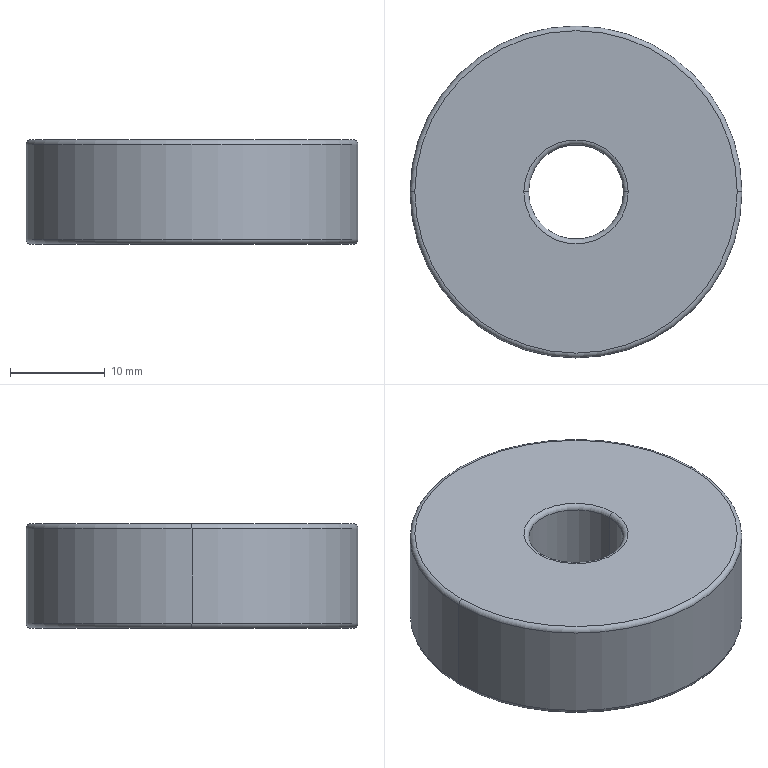Part | STEP file | 6300ZZ | 1 solid | 14 faces | box 35 x 35 x 11 mm | volume 9704 mm3 | torus 8 | cylinder 4 | plane 2 | commonest cylinder face diameters 10 x2 35 x2
STEP:
#1=CARTESIAN_POINT('',(0.,0.,0.));
#2=DIRECTION('',(0.,0.,1.));
#3=DIRECTION('',(1.,0.,0.));
#4=AXIS2_PLACEMENT_3D('',#1,#2,#3);
#5=CARTESIAN_POINT('',(-5.,0.,0.5));
#6=VERTEX_POINT('',#5);
#7=CARTESIAN_POINT('',(5.,0.,0.5));
#8=VERTEX_POINT('',#7);
#9=CARTESIAN_POINT('',(0.,0.,0.5));
#10=DIRECTION('',(0.,0.,-1.));
#11=DIRECTION('',(1.,0.,0.));
#12=AXIS2_PLACEMENT_3D('',#9,#10,#11);
#13=CIRCLE('',#12,5.);
#14=CARTESIAN_POINT('',(0.,0.,0.5));
#15=DIRECTION('',(0.,0.,1.));
#16=DIRECTION('',(1.,0.,0.));
#17=AXIS2_PLACEMENT_3D('',#14,#15,#16);
#18=TOROIDAL_SURFACE('',#17,5.5,0.5);
#19=CARTESIAN_POINT('',(6.283,3.142));
#20=DIRECTION('',(-1.,0.));
#21=VECTOR('',#20,1.);
#22=LINE('',#19,#21);
#23=(GEOMETRIC_REPRESENTATION_CONTEXT(2)PARAMETRIC_REPRESENTATION_CONTEXT()REPRESENTATION_CONTEXT('',''));
#24=DEFINITIONAL_REPRESENTATION('',(#22),#23);
#25=PCURVE('',#18,#24);
#26=CARTESIAN_POINT('',(0.,0.,11.));
#27=DIRECTION('',(0.,0.,-1.));
#28=DIRECTION('',(-1.,0.,0.));
#29=AXIS2_PLACEMENT_3D('',#26,#27,#28);
#30=CYLINDRICAL_SURFACE('',#29,5.);
#31=CARTESIAN_POINT('',(-3.142,10.5));
#32=DIRECTION('',(1.,0.));
#33=VECTOR('',#32,1.);
#34=LINE('',#31,#33);
#35=(GEOMETRIC_REPRESENTATION_CONTEXT(2)PARAMETRIC_REPRESENTATION_CONTEXT()REPRESENTATION_CONTEXT('',''));
#36=DEFINITIONAL_REPRESENTATION('',(#34),#35);
#37=PCURVE('',#30,#36);
#38=SURFACE_CURVE('',#13,(#25,#37),.PCURVE_S1.);
#39=EDGE_CURVE('',#6,#8,#38,.T.);
#40=ORIENTED_EDGE('',*,*,#39,.F.);
#41=CARTESIAN_POINT('',(-5.5,0.,0.));
#42=VERTEX_POINT('',#41);
#43=CARTESIAN_POINT('',(-5.5,0.,0.5));
#44=DIRECTION('',(0.,1.,0.));
#45=DIRECTION('',(-1.,0.,0.));
#46=AXIS2_PLACEMENT_3D('',#43,#44,#45);
#47=CIRCLE('',#46,0.5);
#48=CARTESIAN_POINT('',(3.142,0.));
#49=DIRECTION('',(0.,1.));
#50=VECTOR('',#49,1.);
#51=LINE('',#48,#50);
#52=(GEOMETRIC_REPRESENTATION_CONTEXT(2)PARAMETRIC_REPRESENTATION_CONTEXT()REPRESENTATION_CONTEXT('',''));
#53=DEFINITIONAL_REPRESENTATION('',(#51),#52);
#54=PCURVE('',#18,#53);
#55=CARTESIAN_POINT('',(0.,0.,0.5));
#56=DIRECTION('',(0.,0.,1.));
#57=DIRECTION('',(1.,0.,0.));
#58=AXIS2_PLACEMENT_3D('',#55,#56,#57);
#59=TOROIDAL_SURFACE('',#58,5.5,0.5);
#60=CARTESIAN_POINT('',(3.142,0.));
#61=DIRECTION('',(0.,1.));
#62=VECTOR('',#61,1.);
#63=LINE('',#60,#62);
#64=(GEOMETRIC_REPRESENTATION_CONTEXT(2)PARAMETRIC_REPRESENTATION_CONTEXT()REPRESENTATION_CONTEXT('',''));
#65=DEFINITIONAL_REPRESENTATION('',(#63),#64);
#66=PCURVE('',#59,#65);
#67=SURFACE_CURVE('',#47,(#54,#66),.PCURVE_S1.);
#68=EDGE_CURVE('',#6,#42,#67,.T.);
#69=ORIENTED_EDGE('',*,*,#68,.T.);
#70=CARTESIAN_POINT('',(5.5,0.,0.));
#71=VERTEX_POINT('',#70);
#72=CARTESIAN_POINT('',(0.,0.,0.));
#73=DIRECTION('',(0.,0.,1.));
#74=DIRECTION('',(1.,0.,0.));
#75=AXIS2_PLACEMENT_3D('',#72,#73,#74);
#76=CIRCLE('',#75,5.5);
#77=CARTESIAN_POINT('',(0.,4.712));
#78=DIRECTION('',(1.,0.));
#79=VECTOR('',#78,1.);
#80=LINE('',#77,#79);
#81=(GEOMETRIC_REPRESENTATION_CONTEXT(2)PARAMETRIC_REPRESENTATION_CONTEXT()REPRESENTATION_CONTEXT('',''));
#82=DEFINITIONAL_REPRESENTATION('',(#80),#81);
#83=PCURVE('',#18,#82);
#84=CARTESIAN_POINT('',(0.,0.,0.));
#85=DIRECTION('',(0.,0.,1.));
#86=DIRECTION('',(1.,0.,0.));
#87=AXIS2_PLACEMENT_3D('',#84,#85,#86);
#88=PLANE('',#87);
#89=CARTESIAN_POINT('',(0.,0.));
#90=DIRECTION('',(1.,0.));
#91=AXIS2_PLACEMENT_2D('',#89,#90);
#92=CIRCLE('',#91,5.5);
#93=(GEOMETRIC_REPRESENTATION_CONTEXT(2)PARAMETRIC_REPRESENTATION_CONTEXT()REPRESENTATION_CONTEXT('',''));
#94=DEFINITIONAL_REPRESENTATION('',(#92),#93);
#95=PCURVE('',#88,#94);
#96=SURFACE_CURVE('',#76,(#83,#95),.PCURVE_S1.);
#97=EDGE_CURVE('',#71,#42,#96,.T.);
#98=ORIENTED_EDGE('',*,*,#97,.F.);
#99=CARTESIAN_POINT('',(5.5,0.,0.5));
#100=DIRECTION('',(0.,-1.,0.));
#101=DIRECTION('',(0.,0.,-1.));
#102=AXIS2_PLACEMENT_3D('',#99,#100,#101);
#103=CIRCLE('',#102,0.5);
#104=CARTESIAN_POINT('',(0.,-1.571));
#105=DIRECTION('',(0.,1.));
#106=VECTOR('',#105,1.);
#107=LINE('',#104,#106);
#108=(GEOMETRIC_REPRESENTATION_CONTEXT(2)PARAMETRIC_REPRESENTATION_CONTEXT()REPRESENTATION_CONTEXT('',''));
#109=DEFINITIONAL_REPRESENTATION('',(#107),#108);
#110=PCURVE('',#18,#109);
#111=CARTESIAN_POINT('',(6.283,-1.571));
#112=DIRECTION('',(0.,1.));
#113=VECTOR('',#112,1.);
#114=LINE('',#111,#113);
#115=(GEOMETRIC_REPRESENTATION_CONTEXT(2)PARAMETRIC_REPRESENTATION_CONTEXT()REPRESENTATION_CONTEXT('',''));
#116=DEFINITIONAL_REPRESENTATION('',(#114),#115);
#117=PCURVE('',#59,#116);
#118=SURFACE_CURVE('',#103,(#110,#117),.PCURVE_S1.);
#119=EDGE_CURVE('',#8,#71,#118,.T.);
#120=ORIENTED_EDGE('',*,*,#119,.F.);
#121=EDGE_LOOP('',(#40,#69,#98,#120));
#122=FACE_BOUND('',#121,.T.);
#123=ADVANCED_FACE('',(#122),#18,.T.);
#124=CARTESIAN_POINT('',(-5.5,0.,11.));
#125=VERTEX_POINT('',#124);
#126=CARTESIAN_POINT('',(5.5,0.,11.));
#127=VERTEX_POINT('',#126);
#128=CARTESIAN_POINT('',(0.,0.,11.));
#129=DIRECTION('',(0.,0.,-1.));
#130=DIRECTION('',(1.,0.,0.));
#131=AXIS2_PLACEMENT_3D('',#128,#129,#130);
#132=CIRCLE('',#131,5.5);
#133=CARTESIAN_POINT('',(0.,0.,10.5));
#134=DIRECTION('',(0.,0.,1.));
#135=DIRECTION('',(1.,0.,0.));
#136=AXIS2_PLACEMENT_3D('',#133,#134,#135);
#137=TOROIDAL_SURFACE('',#136,5.5,0.5);
#138=CARTESIAN_POINT('',(6.283,1.571));
#139=DIRECTION('',(-1.,0.));
#140=VECTOR('',#139,1.);
#141=LINE('',#138,#140);
#142=(GEOMETRIC_REPRESENTATION_CONTEXT(2)PARAMETRIC_REPRESENTATION_CONTEXT()REPRESENTATION_CONTEXT('',''));
#143=DEFINITIONAL_REPRESENTATION('',(#141),#142);
#144=PCURVE('',#137,#143);
#145=CARTESIAN_POINT('',(0.,0.,11.));
#146=DIRECTION('',(0.,0.,1.));
#147=DIRECTION('',(1.,0.,0.));
#148=AXIS2_PLACEMENT_3D('',#145,#146,#147);
#149=PLANE('',#148);
#150=CARTESIAN_POINT('',(5.5,0.));
#151=CARTESIAN_POINT('',(5.5,-9.526));
#152=CARTESIAN_POINT('',(-2.75,-4.763));
#153=CARTESIAN_POINT('',(-11.,0.));
#154=CARTESIAN_POINT('',(-2.75,4.763));
#155=CARTESIAN_POINT('',(5.5,9.526));
#156=CARTESIAN_POINT('',(5.5,0.));
#157=(BOUNDED_CURVE()B_SPLINE_CURVE(2,(#150,#151,#152,#153,#154,#155,#156),.UNSPECIFIED.,.T.,.F.)B_SPLINE_CURVE_WITH_KNOTS((1,2,2,2,2,1),(-2.094,0.,2.094,4.189,6.283,8.378),.UNSPECIFIED.)CURVE()GEOMETRIC_REPRESENTATION_ITEM()RATIONAL_B_SPLINE_CURVE((1.,0.5,1.,0.5,1.,0.5,1.))REPRESENTATION_ITEM(''));
#158=(GEOMETRIC_REPRESENTATION_CONTEXT(2)PARAMETRIC_REPRESENTATION_CONTEXT()REPRESENTATION_CONTEXT('',''));
#159=DEFINITIONAL_REPRESENTATION('',(#157),#158);
#160=PCURVE('',#149,#159);
#161=SURFACE_CURVE('',#132,(#144,#160),.PCURVE_S1.);
#162=EDGE_CURVE('',#125,#127,#161,.T.);
#163=ORIENTED_EDGE('',*,*,#162,.F.);
#164=CARTESIAN_POINT('',(-5.,0.,10.5));
#165=VERTEX_POINT('',#164);
#166=CARTESIAN_POINT('',(-5.5,0.,10.5));
#167=DIRECTION('',(0.,1.,0.));
#168=DIRECTION('',(-1.,0.,0.));
#169=AXIS2_PLACEMENT_3D('',#166,#167,#168);
#170=CIRCLE('',#169,0.5);
#171=CARTESIAN_POINT('',(3.142,0.));
#172=DIRECTION('',(0.,1.));
#173=VECTOR('',#172,1.);
#174=LINE('',#171,#173);
#175=(GEOMETRIC_REPRESENTATION_CONTEXT(2)PARAMETRIC_REPRESENTATION_CONTEXT()REPRESENTATION_CONTEXT('',''));
#176=DEFINITIONAL_REPRESENTATION('',(#174),#175);
#177=PCURVE('',#137,#176);
#178=CARTESIAN_POINT('',(0.,0.,10.5));
#179=DIRECTION('',(0.,0.,1.));
#180=DIRECTION('',(1.,0.,0.));
#181=AXIS2_PLACEMENT_3D('',#178,#179,#180);
#182=TOROIDAL_SURFACE('',#181,5.5,0.5);
#183=CARTESIAN_POINT('',(3.142,0.));
#184=DIRECTION('',(0.,1.));
#185=VECTOR('',#184,1.);
#186=LINE('',#183,#185);
#187=(GEOMETRIC_REPRESENTATION_CONTEXT(2)PARAMETRIC_REPRESENTATION_CONTEXT()REPRESENTATION_CONTEXT('',''));
#188=DEFINITIONAL_REPRESENTATION('',(#186),#187);
#189=PCURVE('',#182,#188);
#190=SURFACE_CURVE('',#170,(#177,#189),.PCURVE_S1.);
#191=EDGE_CURVE('',#125,#165,#190,.T.);
#192=ORIENTED_EDGE('',*,*,#191,.T.);
#193=CARTESIAN_POINT('',(5.,0.,10.5));
#194=VERTEX_POINT('',#193);
#195=CARTESIAN_POINT('',(0.,0.,10.5));
#196=DIRECTION('',(0.,0.,1.));
#197=DIRECTION('',(1.,0.,0.));
#198=AXIS2_PLACEMENT_3D('',#195,#196,#197);
#199=CIRCLE('',#198,5.);
#200=CARTESIAN_POINT('',(0.,3.142));
#201=DIRECTION('',(1.,0.));
#202=VECTOR('',#201,1.);
#203=LINE('',#200,#202);
#204=(GEOMETRIC_REPRESENTATION_CONTEXT(2)PARAMETRIC_REPRESENTATION_CONTEXT()REPRESENTATION_CONTEXT('',''));
#205=DEFINITIONAL_REPRESENTATION('',(#203),#204);
#206=PCURVE('',#137,#205);
#207=CARTESIAN_POINT('',(3.142,0.5));
#208=DIRECTION('',(-1.,0.));
#209=VECTOR('',#208,1.);
#210=LINE('',#207,#209);
#211=(GEOMETRIC_REPRESENTATION_CONTEXT(2)PARAMETRIC_REPRESENTATION_CONTEXT()REPRESENTATION_CONTEXT('',''));
#212=DEFINITIONAL_REPRESENTATION('',(#210),#211);
#213=PCURVE('',#30,#212);
#214=SURFACE_CURVE('',#199,(#206,#213),.PCURVE_S1.);
#215=EDGE_CURVE('',#194,#165,#214,.T.);
#216=ORIENTED_EDGE('',*,*,#215,.F.);
#217=CARTESIAN_POINT('',(5.5,0.,10.5));
#218=DIRECTION('',(0.,-1.,0.));
#219=DIRECTION('',(0.,0.,-1.));
#220=AXIS2_PLACEMENT_3D('',#217,#218,#219);
#221=CIRCLE('',#220,0.5);
#222=CARTESIAN_POINT('',(0.,-1.571));
#223=DIRECTION('',(0.,1.));
#224=VECTOR('',#223,1.);
#225=LINE('',#222,#224);
#226=(GEOMETRIC_REPRESENTATION_CONTEXT(2)PARAMETRIC_REPRESENTATION_CONTEXT()REPRESENTATION_CONTEXT('',''));
#227=DEFINITIONAL_REPRESENTATION('',(#225),#226);
#228=PCURVE('',#137,#227);
#229=CARTESIAN_POINT('',(6.283,-1.571));
#230=DIRECTION('',(0.,1.));
#231=VECTOR('',#230,1.);
#232=LINE('',#229,#231);
#233=(GEOMETRIC_REPRESENTATION_CONTEXT(2)PARAMETRIC_REPRESENTATION_CONTEXT()REPRESENTATION_CONTEXT('',''));
#234=DEFINITIONAL_REPRESENTATION('',(#232),#233);
#235=PCURVE('',#182,#234);
#236=SURFACE_CURVE('',#221,(#228,#235),.PCURVE_S1.);
#237=EDGE_CURVE('',#127,#194,#236,.T.);
#238=ORIENTED_EDGE('',*,*,#237,.F.);
#239=EDGE_LOOP('',(#163,#192,#216,#238));
#240=FACE_BOUND('',#239,.T.);
#241=ADVANCED_FACE('',(#240),#137,.T.);
#242=CARTESIAN_POINT('',(-17.5,0.,10.5));
#243=VERTEX_POINT('',#242);
#244=CARTESIAN_POINT('',(17.5,0.,10.5));
#245=VERTEX_POINT('',#244);
#246=CARTESIAN_POINT('',(0.,0.,10.5));
#247=DIRECTION('',(0.,0.,-1.));
#248=DIRECTION('',(1.,0.,0.));
#249=AXIS2_PLACEMENT_3D('',#246,#247,#248);
#250=CIRCLE('',#249,17.5);
#251=CARTESIAN_POINT('',(0.,0.,10.5));
#252=DIRECTION('',(0.,0.,1.));
#253=DIRECTION('',(1.,0.,0.));
#254=AXIS2_PLACEMENT_3D('',#251,#252,#253);
#255=TOROIDAL_SURFACE('',#254,17.,0.5);
#256=CARTESIAN_POINT('',(6.283,0.));
#257=DIRECTION('',(-1.,0.));
#258=VECTOR('',#257,1.);
#259=LINE('',#256,#258);
#260=(GEOMETRIC_REPRESENTATION_CONTEXT(2)PARAMETRIC_REPRESENTATION_CONTEXT()REPRESENTATION_CONTEXT('',''));
#261=DEFINITIONAL_REPRESENTATION('',(#259),#260);
#262=PCURVE('',#255,#261);
#263=CARTESIAN_POINT('',(0.,0.,11.));
#264=DIRECTION('',(0.,0.,-1.));
#265=DIRECTION('',(-1.,0.,0.));
#266=AXIS2_PLACEMENT_3D('',#263,#264,#265);
#267=CYLINDRICAL_SURFACE('',#266,17.5);
#268=CARTESIAN_POINT('',(-3.142,0.5));
#269=DIRECTION('',(1.,0.));
#270=VECTOR('',#269,1.);
#271=LINE('',#268,#270);
#272=(GEOMETRIC_REPRESENTATION_CONTEXT(2)PARAMETRIC_REPRESENTATION_CONTEXT()REPRESENTATION_CONTEXT('',''));
#273=DEFINITIONAL_REPRESENTATION('',(#271),#272);
#274=PCURVE('',#267,#273);
#275=SURFACE_CURVE('',#250,(#262,#274),.PCURVE_S1.);
#276=EDGE_CURVE('',#243,#245,#275,.T.);
#277=ORIENTED_EDGE('',*,*,#276,.F.);
#278=CARTESIAN_POINT('',(-17.,0.,11.));
#279=VERTEX_POINT('',#278);
#280=CARTESIAN_POINT('',(-17.,0.,10.5));
#281=DIRECTION('',(0.,1.,0.));
#282=DIRECTION('',(-1.,0.,0.));
#283=AXIS2_PLACEMENT_3D('',#280,#281,#282);
#284=CIRCLE('',#283,0.5);
#285=CARTESIAN_POINT('',(3.142,0.));
#286=DIRECTION('',(0.,1.));
#287=VECTOR('',#286,1.);
#288=LINE('',#285,#287);
#289=(GEOMETRIC_REPRESENTATION_CONTEXT(2)PARAMETRIC_REPRESENTATION_CONTEXT()REPRESENTATION_CONTEXT('',''));
#290=DEFINITIONAL_REPRESENTATION('',(#288),#289);
#291=PCURVE('',#255,#290);
#292=CARTESIAN_POINT('',(0.,0.,10.5));
#293=DIRECTION('',(0.,0.,1.));
#294=DIRECTION('',(1.,0.,0.));
#295=AXIS2_PLACEMENT_3D('',#292,#293,#294);
#296=TOROIDAL_SURFACE('',#295,17.,0.5);
#297=CARTESIAN_POINT('',(3.142,0.));
#298=DIRECTION('',(0.,1.));
#299=VECTOR('',#298,1.);
#300=LINE('',#297,#299);
#301=(GEOMETRIC_REPRESENTATION_CONTEXT(2)PARAMETRIC_REPRESENTATION_CONTEXT()REPRESENTATION_CONTEXT('',''));
#302=DEFINITIONAL_REPRESENTATION('',(#300),#301);
#303=PCURVE('',#296,#302);
#304=SURFACE_CURVE('',#284,(#291,#303),.PCURVE_S1.);
#305=EDGE_CURVE('',#243,#279,#304,.T.);
#306=ORIENTED_EDGE('',*,*,#305,.T.);
#307=CARTESIAN_POINT('',(17.,0.,11.));
#308=VERTEX_POINT('',#307);
#309=CARTESIAN_POINT('',(0.,0.,11.));
#310=DIRECTION('',(0.,0.,1.));
#311=DIRECTION('',(1.,0.,0.));
#312=AXIS2_PLACEMENT_3D('',#309,#310,#311);
#313=CIRCLE('',#312,17.);
#314=CARTESIAN_POINT('',(0.,1.571));
#315=DIRECTION('',(1.,0.));
#316=VECTOR('',#315,1.);
#317=LINE('',#314,#316);
#318=(GEOMETRIC_REPRESENTATION_CONTEXT(2)PARAMETRIC_REPRESENTATION_CONTEXT()REPRESENTATION_CONTEXT('',''));
#319=DEFINITIONAL_REPRESENTATION('',(#317),#318);
#320=PCURVE('',#255,#319);
#321=CARTESIAN_POINT('',(0.,0.));
#322=DIRECTION('',(1.,0.));
#323=AXIS2_PLACEMENT_2D('',#321,#322);
#324=CIRCLE('',#323,17.);
#325=(GEOMETRIC_REPRESENTATION_CONTEXT(2)PARAMETRIC_REPRESENTATION_CONTEXT()REPRESENTATION_CONTEXT('',''));
#326=DEFINITIONAL_REPRESENTATION('',(#324),#325);
#327=PCURVE('',#149,#326);
#328=SURFACE_CURVE('',#313,(#320,#327),.PCURVE_S1.);
#329=EDGE_CURVE('',#308,#279,#328,.T.);
#330=ORIENTED_EDGE('',*,*,#329,.F.);
#331=CARTESIAN_POINT('',(17.,0.,10.5));
#332=DIRECTION('',(0.,-1.,0.));
#333=DIRECTION('',(0.,0.,-1.));
#334=AXIS2_PLACEMENT_3D('',#331,#332,#333);
#335=CIRCLE('',#334,0.5);
#336=CARTESIAN_POINT('',(0.,-1.571));
#337=DIRECTION('',(0.,1.));
#338=VECTOR('',#337,1.);
#339=LINE('',#336,#338);
#340=(GEOMETRIC_REPRESENTATION_CONTEXT(2)PARAMETRIC_REPRESENTATION_CONTEXT()REPRESENTATION_CONTEXT('',''));
#341=DEFINITIONAL_REPRESENTATION('',(#339),#340);
#342=PCURVE('',#255,#341);
#343=CARTESIAN_POINT('',(6.283,-1.571));
#344=DIRECTION('',(0.,1.));
#345=VECTOR('',#344,1.);
#346=LINE('',#343,#345);
#347=(GEOMETRIC_REPRESENTATION_CONTEXT(2)PARAMETRIC_REPRESENTATION_CONTEXT()REPRESENTATION_CONTEXT('',''));
#348=DEFINITIONAL_REPRESENTATION('',(#346),#347);
#349=PCURVE('',#296,#348);
#350=SURFACE_CURVE('',#335,(#342,#349),.PCURVE_S1.);
#351=EDGE_CURVE('',#245,#308,#350,.T.);
#352=ORIENTED_EDGE('',*,*,#351,.F.);
#353=EDGE_LOOP('',(#277,#306,#330,#352));
#354=FACE_BOUND('',#353,.T.);
#355=ADVANCED_FACE('',(#354),#255,.T.);
#356=CARTESIAN_POINT('',(-17.,0.,0.));
#357=VERTEX_POINT('',#356);
#358=CARTESIAN_POINT('',(17.,0.,0.));
#359=VERTEX_POINT('',#358);
#360=CARTESIAN_POINT('',(0.,0.,0.));
#361=DIRECTION('',(0.,0.,-1.));
#362=DIRECTION('',(1.,0.,0.));
#363=AXIS2_PLACEMENT_3D('',#360,#361,#362);
#364=CIRCLE('',#363,17.);
#365=CARTESIAN_POINT('',(0.,0.,0.5));
#366=DIRECTION('',(0.,0.,1.));
#367=DIRECTION('',(1.,0.,0.));
#368=AXIS2_PLACEMENT_3D('',#365,#366,#367);
#369=TOROIDAL_SURFACE('',#368,17.,0.5);
#370=CARTESIAN_POINT('',(6.283,4.712));
#371=DIRECTION('',(-1.,0.));
#372=VECTOR('',#371,1.);
#373=LINE('',#370,#372);
#374=(GEOMETRIC_REPRESENTATION_CONTEXT(2)PARAMETRIC_REPRESENTATION_CONTEXT()REPRESENTATION_CONTEXT('',''));
#375=DEFINITIONAL_REPRESENTATION('',(#373),#374);
#376=PCURVE('',#369,#375);
#377=CARTESIAN_POINT('',(17.,0.));
#378=CARTESIAN_POINT('',(17.,-29.445));
#379=CARTESIAN_POINT('',(-8.5,-14.722));
#380=CARTESIAN_POINT('',(-34.,0.));
#381=CARTESIAN_POINT('',(-8.5,14.722));
#382=CARTESIAN_POINT('',(17.,29.445));
#383=CARTESIAN_POINT('',(17.,0.));
#384=(BOUNDED_CURVE()B_SPLINE_CURVE(2,(#377,#378,#379,#380,#381,#382,#383),.UNSPECIFIED.,.T.,.F.)B_SPLINE_CURVE_WITH_KNOTS((1,2,2,2,2,1),(-2.094,0.,2.094,4.189,6.283,8.378),.UNSPECIFIED.)CURVE()GEOMETRIC_REPRESENTATION_ITEM()RATIONAL_B_SPLINE_CURVE((1.,0.5,1.,0.5,1.,0.5,1.))REPRESENTATION_ITEM(''));
#385=(GEOMETRIC_REPRESENTATION_CONTEXT(2)PARAMETRIC_REPRESENTATION_CONTEXT()REPRESENTATION_CONTEXT('',''));
#386=DEFINITIONAL_REPRESENTATION('',(#384),#385);
#387=PCURVE('',#88,#386);
#388=SURFACE_CURVE('',#364,(#376,#387),.PCURVE_S1.);
#389=EDGE_CURVE('',#357,#359,#388,.T.);
#390=ORIENTED_EDGE('',*,*,#389,.F.);
#391=CARTESIAN_POINT('',(-17.5,0.,0.5));
#392=VERTEX_POINT('',#391);
#393=CARTESIAN_POINT('',(-17.,0.,0.5));
#394=DIRECTION('',(0.,1.,0.));
#395=DIRECTION('',(-1.,0.,0.));
#396=AXIS2_PLACEMENT_3D('',#393,#394,#395);
#397=CIRCLE('',#396,0.5);
#398=CARTESIAN_POINT('',(3.142,0.));
#399=DIRECTION('',(0.,1.));
#400=VECTOR('',#399,1.);
#401=LINE('',#398,#400);
#402=(GEOMETRIC_REPRESENTATION_CONTEXT(2)PARAMETRIC_REPRESENTATION_CONTEXT()REPRESENTATION_CONTEXT('',''));
#403=DEFINITIONAL_REPRESENTATION('',(#401),#402);
#404=PCURVE('',#369,#403);
#405=CARTESIAN_POINT('',(0.,0.,0.5));
#406=DIRECTION('',(0.,0.,1.));
#407=DIRECTION('',(1.,0.,0.));
#408=AXIS2_PLACEMENT_3D('',#405,#406,#407);
#409=TOROIDAL_SURFACE('',#408,17.,0.5);
#410=CARTESIAN_POINT('',(3.142,0.));
#411=DIRECTION('',(0.,1.));
#412=VECTOR('',#411,1.);
#413=LINE('',#410,#412);
#414=(GEOMETRIC_REPRESENTATION_CONTEXT(2)PARAMETRIC_REPRESENTATION_CONTEXT()REPRESENTATION_CONTEXT('',''));
#415=DEFINITIONAL_REPRESENTATION('',(#413),#414);
#416=PCURVE('',#409,#415);
#417=SURFACE_CURVE('',#397,(#404,#416),.PCURVE_S1.);
#418=EDGE_CURVE('',#357,#392,#417,.T.);
#419=ORIENTED_EDGE('',*,*,#418,.T.);
#420=CARTESIAN_POINT('',(17.5,0.,0.5));
#421=VERTEX_POINT('',#420);
#422=CARTESIAN_POINT('',(0.,0.,0.5));
#423=DIRECTION('',(0.,0.,1.));
#424=DIRECTION('',(1.,0.,0.));
#425=AXIS2_PLACEMENT_3D('',#422,#423,#424);
#426=CIRCLE('',#425,17.5);
#427=CARTESIAN_POINT('',(0.,6.283));
#428=DIRECTION('',(1.,0.));
#429=VECTOR('',#428,1.);
#430=LINE('',#427,#429);
#431=(GEOMETRIC_REPRESENTATION_CONTEXT(2)PARAMETRIC_REPRESENTATION_CONTEXT()REPRESENTATION_CONTEXT('',''));
#432=DEFINITIONAL_REPRESENTATION('',(#430),#431);
#433=PCURVE('',#369,#432);
#434=CARTESIAN_POINT('',(3.142,10.5));
#435=DIRECTION('',(-1.,0.));
#436=VECTOR('',#435,1.);
#437=LINE('',#434,#436);
#438=(GEOMETRIC_REPRESENTATION_CONTEXT(2)PARAMETRIC_REPRESENTATION_CONTEXT()REPRESENTATION_CONTEXT('',''));
#439=DEFINITIONAL_REPRESENTATION('',(#437),#438);
#440=PCURVE('',#267,#439);
#441=SURFACE_CURVE('',#426,(#433,#440),.PCURVE_S1.);
#442=EDGE_CURVE('',#421,#392,#441,.T.);
#443=ORIENTED_EDGE('',*,*,#442,.F.);
#444=CARTESIAN_POINT('',(17.,0.,0.5));
#445=DIRECTION('',(0.,-1.,0.));
#446=DIRECTION('',(0.,0.,-1.));
#447=AXIS2_PLACEMENT_3D('',#444,#445,#446);
#448=CIRCLE('',#447,0.5);
#449=CARTESIAN_POINT('',(0.,4.712));
#450=DIRECTION('',(0.,1.));
#451=VECTOR('',#450,1.);
#452=LINE('',#449,#451);
#453=(GEOMETRIC_REPRESENTATION_CONTEXT(2)PARAMETRIC_REPRESENTATION_CONTEXT()REPRESENTATION_CONTEXT('',''));
#454=DEFINITIONAL_REPRESENTATION('',(#452),#453);
#455=PCURVE('',#369,#454);
#456=CARTESIAN_POINT('',(6.283,4.712));
#457=DIRECTION('',(0.,1.));
#458=VECTOR('',#457,1.);
#459=LINE('',#456,#458);
#460=(GEOMETRIC_REPRESENTATION_CONTEXT(2)PARAMETRIC_REPRESENTATION_CONTEXT()REPRESENTATION_CONTEXT('',''));
#461=DEFINITIONAL_REPRESENTATION('',(#459),#460);
#462=PCURVE('',#409,#461);
#463=SURFACE_CURVE('',#448,(#455,#462),.PCURVE_S1.);
#464=EDGE_CURVE('',#359,#421,#463,.T.);
#465=ORIENTED_EDGE('',*,*,#464,.F.);
#466=EDGE_LOOP('',(#390,#419,#443,#465));
#467=FACE_BOUND('',#466,.T.);
#468=ADVANCED_FACE('',(#467),#369,.T.);
#469=CARTESIAN_POINT('',(-5.,0.,11.));
#470=DIRECTION('',(0.,0.,-1.));
#471=VECTOR('',#470,1.);
#472=LINE('',#469,#471);
#473=CARTESIAN_POINT('',(0.,0.,11.));
#474=DIRECTION('',(0.,0.,-1.));
#475=DIRECTION('',(-1.,0.,0.));
#476=AXIS2_PLACEMENT_3D('',#473,#474,#475);
#477=CYLINDRICAL_SURFACE('',#476,5.);
#478=CARTESIAN_POINT('',(6.283,0.));
#479=DIRECTION('',(0.,1.));
#480=VECTOR('',#479,1.);
#481=LINE('',#478,#480);
#482=(GEOMETRIC_REPRESENTATION_CONTEXT(2)PARAMETRIC_REPRESENTATION_CONTEXT()REPRESENTATION_CONTEXT('',''));
#483=DEFINITIONAL_REPRESENTATION('',(#481),#482);
#484=PCURVE('',#477,#483);
#485=CARTESIAN_POINT('',(0.,0.));
#486=DIRECTION('',(0.,1.));
#487=VECTOR('',#486,1.);
#488=LINE('',#485,#487);
#489=(GEOMETRIC_REPRESENTATION_CONTEXT(2)PARAMETRIC_REPRESENTATION_CONTEXT()REPRESENTATION_CONTEXT('',''));
#490=DEFINITIONAL_REPRESENTATION('',(#488),#489);
#491=PCURVE('',#30,#490);
#492=SURFACE_CURVE('',#472,(#484,#491),.PCURVE_S1.);
#493=EDGE_CURVE('',#165,#6,#492,.T.);
#494=ORIENTED_EDGE('',*,*,#493,.T.);
#495=CARTESIAN_POINT('',(0.,0.,0.5));
#496=DIRECTION('',(0.,0.,-1.));
#497=DIRECTION('',(1.,0.,0.));
#498=AXIS2_PLACEMENT_3D('',#495,#496,#497);
#499=CIRCLE('',#498,5.);
#500=CARTESIAN_POINT('',(3.142,10.5));
#501=DIRECTION('',(1.,0.));
#502=VECTOR('',#501,1.);
#503=LINE('',#500,#502);
#504=(GEOMETRIC_REPRESENTATION_CONTEXT(2)PARAMETRIC_REPRESENTATION_CONTEXT()REPRESENTATION_CONTEXT('',''));
#505=DEFINITIONAL_REPRESENTATION('',(#503),#504);
#506=PCURVE('',#477,#505);
#507=CARTESIAN_POINT('',(6.283,3.142));
#508=DIRECTION('',(-1.,0.));
#509=VECTOR('',#508,1.);
#510=LINE('',#507,#509);
#511=(GEOMETRIC_REPRESENTATION_CONTEXT(2)PARAMETRIC_REPRESENTATION_CONTEXT()REPRESENTATION_CONTEXT('',''));
#512=DEFINITIONAL_REPRESENTATION('',(#510),#511);
#513=PCURVE('',#59,#512);
#514=SURFACE_CURVE('',#499,(#506,#513),.PCURVE_S1.);
#515=EDGE_CURVE('',#8,#6,#514,.T.);
#516=ORIENTED_EDGE('',*,*,#515,.F.);
#517=CARTESIAN_POINT('',(5.,0.,11.));
#518=DIRECTION('',(0.,0.,-1.));
#519=VECTOR('',#518,1.);
#520=LINE('',#517,#519);
#521=CARTESIAN_POINT('',(3.142,0.));
#522=DIRECTION('',(0.,1.));
#523=VECTOR('',#522,1.);
#524=LINE('',#521,#523);
#525=(GEOMETRIC_REPRESENTATION_CONTEXT(2)PARAMETRIC_REPRESENTATION_CONTEXT()REPRESENTATION_CONTEXT('',''));
#526=DEFINITIONAL_REPRESENTATION('',(#524),#525);
#527=PCURVE('',#477,#526);
#528=CARTESIAN_POINT('',(3.142,0.));
#529=DIRECTION('',(0.,1.));
#530=VECTOR('',#529,1.);
#531=LINE('',#528,#530);
#532=(GEOMETRIC_REPRESENTATION_CONTEXT(2)PARAMETRIC_REPRESENTATION_CONTEXT()REPRESENTATION_CONTEXT('',''));
#533=DEFINITIONAL_REPRESENTATION('',(#531),#532);
#534=PCURVE('',#30,#533);
#535=SURFACE_CURVE('',#520,(#527,#534),.PCURVE_S1.);
#536=EDGE_CURVE('',#194,#8,#535,.T.);
#537=ORIENTED_EDGE('',*,*,#536,.F.);
#538=CARTESIAN_POINT('',(0.,0.,10.5));
#539=DIRECTION('',(0.,0.,1.));
#540=DIRECTION('',(1.,0.,0.));
#541=AXIS2_PLACEMENT_3D('',#538,#539,#540);
#542=CIRCLE('',#541,5.);
#543=CARTESIAN_POINT('',(9.425,0.5));
#544=DIRECTION('',(-1.,0.));
#545=VECTOR('',#544,1.);
#546=LINE('',#543,#545);
#547=(GEOMETRIC_REPRESENTATION_CONTEXT(2)PARAMETRIC_REPRESENTATION_CONTEXT()REPRESENTATION_CONTEXT('',''));
#548=DEFINITIONAL_REPRESENTATION('',(#546),#547);
#549=PCURVE('',#477,#548);
#550=CARTESIAN_POINT('',(0.,3.142));
#551=DIRECTION('',(1.,0.));
#552=VECTOR('',#551,1.);
#553=LINE('',#550,#552);
#554=(GEOMETRIC_REPRESENTATION_CONTEXT(2)PARAMETRIC_REPRESENTATION_CONTEXT()REPRESENTATION_CONTEXT('',''));
#555=DEFINITIONAL_REPRESENTATION('',(#553),#554);
#556=PCURVE('',#182,#555);
#557=SURFACE_CURVE('',#542,(#549,#556),.PCURVE_S1.);
#558=EDGE_CURVE('',#165,#194,#557,.T.);
#559=ORIENTED_EDGE('',*,*,#558,.F.);
#560=EDGE_LOOP('',(#494,#516,#537,#559));
#561=FACE_BOUND('',#560,.F.);
#562=ADVANCED_FACE('',(#561),#477,.F.);
#563=ORIENTED_EDGE('',*,*,#276,.T.);
#564=CARTESIAN_POINT('',(17.5,0.,11.));
#565=DIRECTION('',(0.,0.,-1.));
#566=VECTOR('',#565,1.);
#567=LINE('',#564,#566);
#568=CARTESIAN_POINT('',(3.142,0.));
#569=DIRECTION('',(0.,1.));
#570=VECTOR('',#569,1.);
#571=LINE('',#568,#570);
#572=(GEOMETRIC_REPRESENTATION_CONTEXT(2)PARAMETRIC_REPRESENTATION_CONTEXT()REPRESENTATION_CONTEXT('',''));
#573=DEFINITIONAL_REPRESENTATION('',(#571),#572);
#574=PCURVE('',#267,#573);
#575=CARTESIAN_POINT('',(0.,0.,11.));
#576=DIRECTION('',(0.,0.,-1.));
#577=DIRECTION('',(-1.,0.,0.));
#578=AXIS2_PLACEMENT_3D('',#575,#576,#577);
#579=CYLINDRICAL_SURFACE('',#578,17.5);
#580=CARTESIAN_POINT('',(3.142,0.));
#581=DIRECTION('',(0.,1.));
#582=VECTOR('',#581,1.);
#583=LINE('',#580,#582);
#584=(GEOMETRIC_REPRESENTATION_CONTEXT(2)PARAMETRIC_REPRESENTATION_CONTEXT()REPRESENTATION_CONTEXT('',''));
#585=DEFINITIONAL_REPRESENTATION('',(#583),#584);
#586=PCURVE('',#579,#585);
#587=SURFACE_CURVE('',#567,(#574,#586),.PCURVE_S1.);
#588=EDGE_CURVE('',#245,#421,#587,.T.);
#589=ORIENTED_EDGE('',*,*,#588,.T.);
#590=ORIENTED_EDGE('',*,*,#442,.T.);
#591=CARTESIAN_POINT('',(-17.5,0.,11.));
#592=DIRECTION('',(0.,0.,-1.));
#593=VECTOR('',#592,1.);
#594=LINE('',#591,#593);
#595=CARTESIAN_POINT('',(0.,0.));
#596=DIRECTION('',(0.,1.));
#597=VECTOR('',#596,1.);
#598=LINE('',#595,#597);
#599=(GEOMETRIC_REPRESENTATION_CONTEXT(2)PARAMETRIC_REPRESENTATION_CONTEXT()REPRESENTATION_CONTEXT('',''));
#600=DEFINITIONAL_REPRESENTATION('',(#598),#599);
#601=PCURVE('',#267,#600);
#602=CARTESIAN_POINT('',(6.283,0.));
#603=DIRECTION('',(0.,1.));
#604=VECTOR('',#603,1.);
#605=LINE('',#602,#604);
#606=(GEOMETRIC_REPRESENTATION_CONTEXT(2)PARAMETRIC_REPRESENTATION_CONTEXT()REPRESENTATION_CONTEXT('',''));
#607=DEFINITIONAL_REPRESENTATION('',(#605),#606);
#608=PCURVE('',#579,#607);
#609=SURFACE_CURVE('',#594,(#601,#608),.PCURVE_S1.);
#610=EDGE_CURVE('',#243,#392,#609,.T.);
#611=ORIENTED_EDGE('',*,*,#610,.F.);
#612=EDGE_LOOP('',(#563,#589,#590,#611));
#613=FACE_BOUND('',#612,.T.);
#614=ADVANCED_FACE('',(#613),#267,.T.);
#615=ORIENTED_EDGE('',*,*,#329,.T.);
#616=CARTESIAN_POINT('',(0.,0.,11.));
#617=DIRECTION('',(0.,0.,1.));
#618=DIRECTION('',(1.,0.,0.));
#619=AXIS2_PLACEMENT_3D('',#616,#617,#618);
#620=CIRCLE('',#619,17.);
#621=CARTESIAN_POINT('',(0.,0.));
#622=DIRECTION('',(1.,0.));
#623=AXIS2_PLACEMENT_2D('',#621,#622);
#624=CIRCLE('',#623,17.);
#625=(GEOMETRIC_REPRESENTATION_CONTEXT(2)PARAMETRIC_REPRESENTATION_CONTEXT()REPRESENTATION_CONTEXT('',''));
#626=DEFINITIONAL_REPRESENTATION('',(#624),#625);
#627=PCURVE('',#149,#626);
#628=CARTESIAN_POINT('',(0.,1.571));
#629=DIRECTION('',(1.,0.));
#630=VECTOR('',#629,1.);
#631=LINE('',#628,#630);
#632=(GEOMETRIC_REPRESENTATION_CONTEXT(2)PARAMETRIC_REPRESENTATION_CONTEXT()REPRESENTATION_CONTEXT('',''));
#633=DEFINITIONAL_REPRESENTATION('',(#631),#632);
#634=PCURVE('',#296,#633);
#635=SURFACE_CURVE('',#620,(#627,#634),.PCURVE_S1.);
#636=EDGE_CURVE('',#279,#308,#635,.T.);
#637=ORIENTED_EDGE('',*,*,#636,.T.);
#638=EDGE_LOOP('',(#615,#637));
#639=FACE_BOUND('',#638,.T.);
#640=CARTESIAN_POINT('',(0.,0.,11.));
#641=DIRECTION('',(0.,0.,-1.));
#642=DIRECTION('',(1.,0.,0.));
#643=AXIS2_PLACEMENT_3D('',#640,#641,#642);
#644=CIRCLE('',#643,5.5);
#645=CARTESIAN_POINT('',(5.5,0.));
#646=CARTESIAN_POINT('',(5.5,-9.526));
#647=CARTESIAN_POINT('',(-2.75,-4.763));
#648=CARTESIAN_POINT('',(-11.,0.));
#649=CARTESIAN_POINT('',(-2.75,4.763));
#650=CARTESIAN_POINT('',(5.5,9.526));
#651=CARTESIAN_POINT('',(5.5,0.));
#652=(BOUNDED_CURVE()B_SPLINE_CURVE(2,(#645,#646,#647,#648,#649,#650,#651),.UNSPECIFIED.,.T.,.F.)B_SPLINE_CURVE_WITH_KNOTS((1,2,2,2,2,1),(-2.094,0.,2.094,4.189,6.283,8.378),.UNSPECIFIED.)CURVE()GEOMETRIC_REPRESENTATION_ITEM()RATIONAL_B_SPLINE_CURVE((1.,0.5,1.,0.5,1.,0.5,1.))REPRESENTATION_ITEM(''));
#653=(GEOMETRIC_REPRESENTATION_CONTEXT(2)PARAMETRIC_REPRESENTATION_CONTEXT()REPRESENTATION_CONTEXT('',''));
#654=DEFINITIONAL_REPRESENTATION('',(#652),#653);
#655=PCURVE('',#149,#654);
#656=CARTESIAN_POINT('',(6.283,1.571));
#657=DIRECTION('',(-1.,0.));
#658=VECTOR('',#657,1.);
#659=LINE('',#656,#658);
#660=(GEOMETRIC_REPRESENTATION_CONTEXT(2)PARAMETRIC_REPRESENTATION_CONTEXT()REPRESENTATION_CONTEXT('',''));
#661=DEFINITIONAL_REPRESENTATION('',(#659),#660);
#662=PCURVE('',#182,#661);
#663=SURFACE_CURVE('',#644,(#655,#662),.PCURVE_S1.);
#664=EDGE_CURVE('',#127,#125,#663,.T.);
#665=ORIENTED_EDGE('',*,*,#664,.T.);
#666=ORIENTED_EDGE('',*,*,#162,.T.);
#667=EDGE_LOOP('',(#665,#666));
#668=FACE_BOUND('',#667,.T.);
#669=ADVANCED_FACE('',(#639,#668),#149,.T.);
#670=CARTESIAN_POINT('',(0.,0.,0.));
#671=DIRECTION('',(0.,0.,-1.));
#672=DIRECTION('',(1.,0.,0.));
#673=AXIS2_PLACEMENT_3D('',#670,#671,#672);
#674=CIRCLE('',#673,17.);
#675=CARTESIAN_POINT('',(17.,0.));
#676=CARTESIAN_POINT('',(17.,-29.445));
#677=CARTESIAN_POINT('',(-8.5,-14.722));
#678=CARTESIAN_POINT('',(-34.,0.));
#679=CARTESIAN_POINT('',(-8.5,14.722));
#680=CARTESIAN_POINT('',(17.,29.445));
#681=CARTESIAN_POINT('',(17.,0.));
#682=(BOUNDED_CURVE()B_SPLINE_CURVE(2,(#675,#676,#677,#678,#679,#680,#681),.UNSPECIFIED.,.T.,.F.)B_SPLINE_CURVE_WITH_KNOTS((1,2,2,2,2,1),(-2.094,0.,2.094,4.189,6.283,8.378),.UNSPECIFIED.)CURVE()GEOMETRIC_REPRESENTATION_ITEM()RATIONAL_B_SPLINE_CURVE((1.,0.5,1.,0.5,1.,0.5,1.))REPRESENTATION_ITEM(''));
#683=(GEOMETRIC_REPRESENTATION_CONTEXT(2)PARAMETRIC_REPRESENTATION_CONTEXT()REPRESENTATION_CONTEXT('',''));
#684=DEFINITIONAL_REPRESENTATION('',(#682),#683);
#685=PCURVE('',#88,#684);
#686=CARTESIAN_POINT('',(6.283,4.712));
#687=DIRECTION('',(-1.,0.));
#688=VECTOR('',#687,1.);
#689=LINE('',#686,#688);
#690=(GEOMETRIC_REPRESENTATION_CONTEXT(2)PARAMETRIC_REPRESENTATION_CONTEXT()REPRESENTATION_CONTEXT('',''));
#691=DEFINITIONAL_REPRESENTATION('',(#689),#690);
#692=PCURVE('',#409,#691);
#693=SURFACE_CURVE('',#674,(#685,#692),.PCURVE_S1.);
#694=EDGE_CURVE('',#359,#357,#693,.T.);
#695=ORIENTED_EDGE('',*,*,#694,.T.);
#696=ORIENTED_EDGE('',*,*,#389,.T.);
#697=EDGE_LOOP('',(#695,#696));
#698=FACE_BOUND('',#697,.T.);
#699=ORIENTED_EDGE('',*,*,#97,.T.);
#700=CARTESIAN_POINT('',(0.,0.,0.));
#701=DIRECTION('',(0.,0.,1.));
#702=DIRECTION('',(1.,0.,0.));
#703=AXIS2_PLACEMENT_3D('',#700,#701,#702);
#704=CIRCLE('',#703,5.5);
#705=CARTESIAN_POINT('',(0.,0.));
#706=DIRECTION('',(1.,0.));
#707=AXIS2_PLACEMENT_2D('',#705,#706);
#708=CIRCLE('',#707,5.5);
#709=(GEOMETRIC_REPRESENTATION_CONTEXT(2)PARAMETRIC_REPRESENTATION_CONTEXT()REPRESENTATION_CONTEXT('',''));
#710=DEFINITIONAL_REPRESENTATION('',(#708),#709);
#711=PCURVE('',#88,#710);
#712=CARTESIAN_POINT('',(0.,4.712));
#713=DIRECTION('',(1.,0.));
#714=VECTOR('',#713,1.);
#715=LINE('',#712,#714);
#716=(GEOMETRIC_REPRESENTATION_CONTEXT(2)PARAMETRIC_REPRESENTATION_CONTEXT()REPRESENTATION_CONTEXT('',''));
#717=DEFINITIONAL_REPRESENTATION('',(#715),#716);
#718=PCURVE('',#59,#717);
#719=SURFACE_CURVE('',#704,(#711,#718),.PCURVE_S1.);
#720=EDGE_CURVE('',#42,#71,#719,.T.);
#721=ORIENTED_EDGE('',*,*,#720,.T.);
#722=EDGE_LOOP('',(#699,#721));
#723=FACE_BOUND('',#722,.T.);
#724=ADVANCED_FACE('',(#698,#723),#88,.F.);
#725=ORIENTED_EDGE('',*,*,#588,.F.);
#726=CARTESIAN_POINT('',(0.,0.,10.5));
#727=DIRECTION('',(0.,0.,-1.));
#728=DIRECTION('',(1.,0.,0.));
#729=AXIS2_PLACEMENT_3D('',#726,#727,#728);
#730=CIRCLE('',#729,17.5);
#731=CARTESIAN_POINT('',(3.142,0.5));
#732=DIRECTION('',(1.,0.));
#733=VECTOR('',#732,1.);
#734=LINE('',#731,#733);
#735=(GEOMETRIC_REPRESENTATION_CONTEXT(2)PARAMETRIC_REPRESENTATION_CONTEXT()REPRESENTATION_CONTEXT('',''));
#736=DEFINITIONAL_REPRESENTATION('',(#734),#735);
#737=PCURVE('',#579,#736);
#738=CARTESIAN_POINT('',(6.283,0.));
#739=DIRECTION('',(-1.,0.));
#740=VECTOR('',#739,1.);
#741=LINE('',#738,#740);
#742=(GEOMETRIC_REPRESENTATION_CONTEXT(2)PARAMETRIC_REPRESENTATION_CONTEXT()REPRESENTATION_CONTEXT('',''));
#743=DEFINITIONAL_REPRESENTATION('',(#741),#742);
#744=PCURVE('',#296,#743);
#745=SURFACE_CURVE('',#730,(#737,#744),.PCURVE_S1.);
#746=EDGE_CURVE('',#245,#243,#745,.T.);
#747=ORIENTED_EDGE('',*,*,#746,.T.);
#748=ORIENTED_EDGE('',*,*,#610,.T.);
#749=CARTESIAN_POINT('',(0.,0.,0.5));
#750=DIRECTION('',(0.,0.,1.));
#751=DIRECTION('',(1.,0.,0.));
#752=AXIS2_PLACEMENT_3D('',#749,#750,#751);
#753=CIRCLE('',#752,17.5);
#754=CARTESIAN_POINT('',(9.425,10.5));
#755=DIRECTION('',(-1.,0.));
#756=VECTOR('',#755,1.);
#757=LINE('',#754,#756);
#758=(GEOMETRIC_REPRESENTATION_CONTEXT(2)PARAMETRIC_REPRESENTATION_CONTEXT()REPRESENTATION_CONTEXT('',''));
#759=DEFINITIONAL_REPRESENTATION('',(#757),#758);
#760=PCURVE('',#579,#759);
#761=CARTESIAN_POINT('',(0.,6.283));
#762=DIRECTION('',(1.,0.));
#763=VECTOR('',#762,1.);
#764=LINE('',#761,#763);
#765=(GEOMETRIC_REPRESENTATION_CONTEXT(2)PARAMETRIC_REPRESENTATION_CONTEXT()REPRESENTATION_CONTEXT('',''));
#766=DEFINITIONAL_REPRESENTATION('',(#764),#765);
#767=PCURVE('',#409,#766);
#768=SURFACE_CURVE('',#753,(#760,#767),.PCURVE_S1.);
#769=EDGE_CURVE('',#392,#421,#768,.T.);
#770=ORIENTED_EDGE('',*,*,#769,.T.);
#771=EDGE_LOOP('',(#725,#747,#748,#770));
#772=FACE_BOUND('',#771,.T.);
#773=ADVANCED_FACE('',(#772),#579,.T.);
#774=ORIENTED_EDGE('',*,*,#39,.F.);
#775=ORIENTED_EDGE('',*,*,#493,.F.);
#776=ORIENTED_EDGE('',*,*,#215,.F.);
#777=ORIENTED_EDGE('',*,*,#536,.T.);
#778=EDGE_LOOP('',(#774,#775,#776,#777));
#779=FACE_BOUND('',#778,.F.);
#780=ADVANCED_FACE('',(#779),#30,.F.);
#781=ORIENTED_EDGE('',*,*,#418,.F.);
#782=ORIENTED_EDGE('',*,*,#694,.F.);
#783=ORIENTED_EDGE('',*,*,#464,.T.);
#784=ORIENTED_EDGE('',*,*,#769,.F.);
#785=EDGE_LOOP('',(#781,#782,#783,#784));
#786=FACE_BOUND('',#785,.T.);
#787=ADVANCED_FACE('',(#786),#409,.T.);
#788=ORIENTED_EDGE('',*,*,#305,.F.);
#789=ORIENTED_EDGE('',*,*,#746,.F.);
#790=ORIENTED_EDGE('',*,*,#351,.T.);
#791=ORIENTED_EDGE('',*,*,#636,.F.);
#792=EDGE_LOOP('',(#788,#789,#790,#791));
#793=FACE_BOUND('',#792,.T.);
#794=ADVANCED_FACE('',(#793),#296,.T.);
#795=ORIENTED_EDGE('',*,*,#191,.F.);
#796=ORIENTED_EDGE('',*,*,#664,.F.);
#797=ORIENTED_EDGE('',*,*,#237,.T.);
#798=ORIENTED_EDGE('',*,*,#558,.F.);
#799=EDGE_LOOP('',(#795,#796,#797,#798));
#800=FACE_BOUND('',#799,.T.);
#801=ADVANCED_FACE('',(#800),#182,.T.);
#802=ORIENTED_EDGE('',*,*,#68,.F.);
#803=ORIENTED_EDGE('',*,*,#515,.F.);
#804=ORIENTED_EDGE('',*,*,#119,.T.);
#805=ORIENTED_EDGE('',*,*,#720,.F.);
#806=EDGE_LOOP('',(#802,#803,#804,#805));
#807=FACE_BOUND('',#806,.T.);
#808=ADVANCED_FACE('',(#807),#59,.T.);
#809=CLOSED_SHELL('',(#123,#241,#355,#468,#562,#614,#669,#724,#773,#780,#787,#794,#801,#808));
#810=MANIFOLD_SOLID_BREP('',#809);
#811=(LENGTH_UNIT()NAMED_UNIT(*)SI_UNIT(.MILLI.,.METRE.));
#812=UNCERTAINTY_MEASURE_WITH_UNIT(LENGTH_MEASURE(0.0000001),#811,'','');
#813=(NAMED_UNIT(*)PLANE_ANGLE_UNIT()SI_UNIT($,.RADIAN.));
#814=(NAMED_UNIT(*)SI_UNIT($,.STERADIAN.)SOLID_ANGLE_UNIT());
#815=(GEOMETRIC_REPRESENTATION_CONTEXT(3)GLOBAL_UNCERTAINTY_ASSIGNED_CONTEXT((#812))GLOBAL_UNIT_ASSIGNED_CONTEXT((#811,#813,#814))REPRESENTATION_CONTEXT('',''));
#816=ADVANCED_BREP_SHAPE_REPRESENTATION('',(#4,#810),#815);